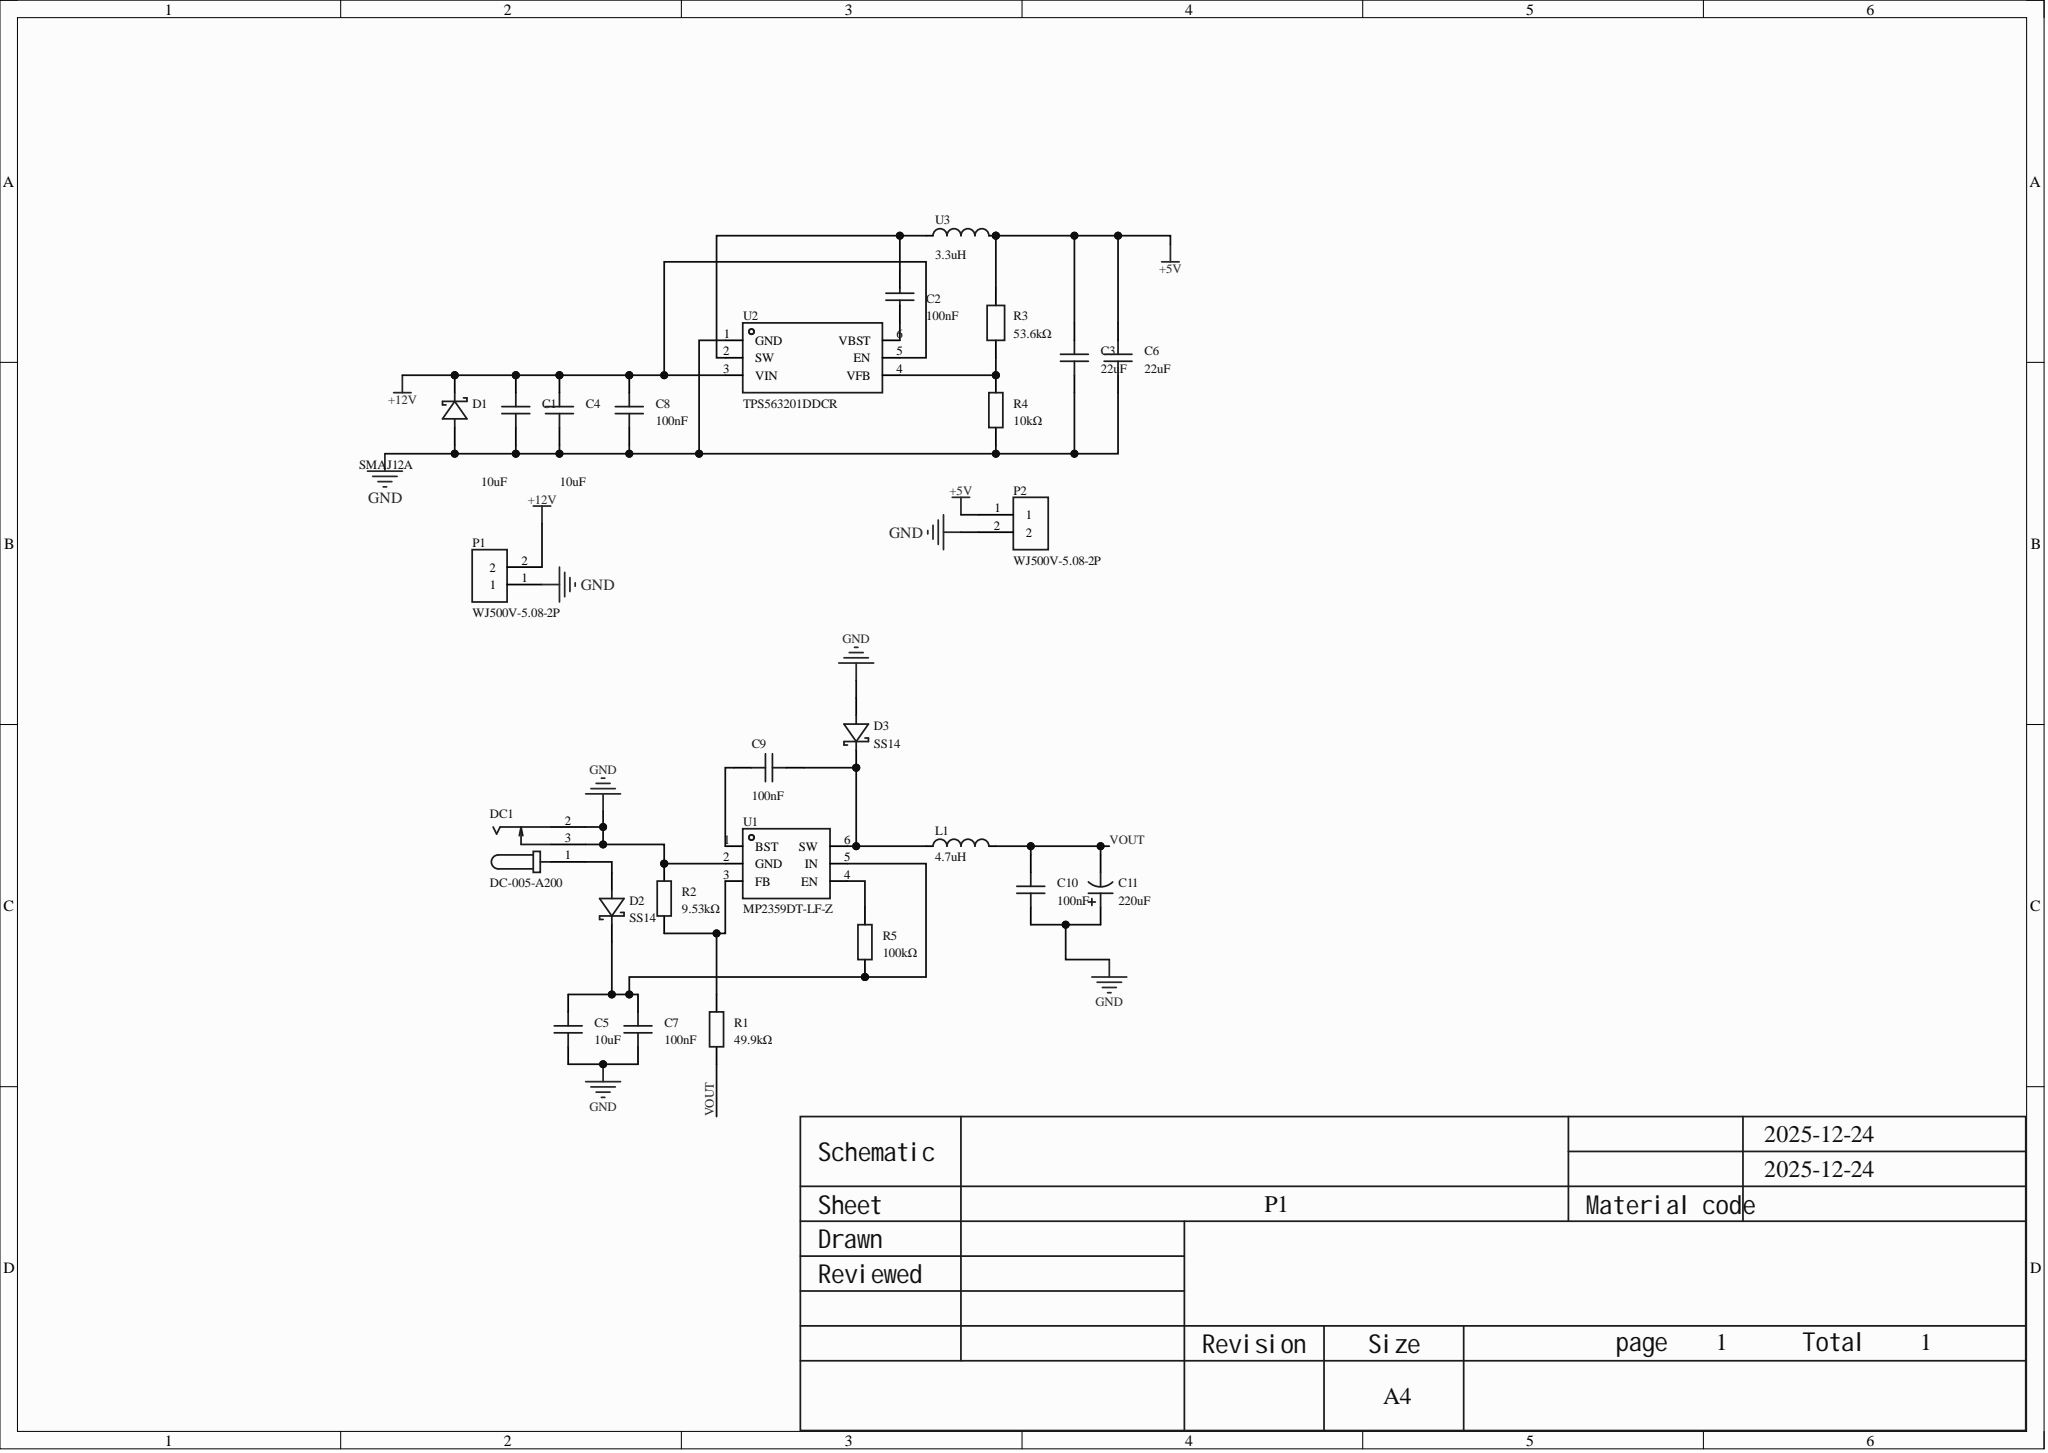Circuit board | Altium Designer | 26 parts | 13 nets
Bill of materials:
Comment,Description,Designator,Footprint,LibRef,Quantity
"10uF","Capacitance: 10uF; Tolerance: ±10%; Rated voltage: 35V; Dielectric (temp. coefficient): X5R;","C1, C4","C0805","CGA0805X5R106K350MT","2"
"100nF","Capacitance: 100nF; Tolerance: ±10%; Rated voltage: 25V; Dielectric (temp. coefficient): X7R;, Capacitance: 100nF; Tolerance: ±10%; Rated voltage: 50V; Dielectric (temp. coefficient): X7R;","C2, C7, C8, C9, C10","C0603","CL10B104KA8NNNC, CGA0603X7R104K500JT","5"
"22uF","Capacitance: 22uF; Tolerance: ±20%; Rated voltage: 10V; Dielectric (temp. coefficient): X5R;","C3, C6","C0603","HGC0603R5226M100NTHJ","2"
"10uF","Capacitance: 10uF; Tolerance: ±10%; Rated voltage: 10V; Dielectric (temp. coefficient): X5R;","C5","C0603","CGA0603X5R106K100JT","1"
"220uF","Capacitance: 220uF; Tolerance: ±20%; Rated voltage: 50V; Ripple current: 220mA@120Hz;","C11","CAP-SMD_BD10.0-L10.3-W10.3-LS11.7-FD","JVJ50V220M10x10","1"
"SMAJ12A","Reverse standoff voltage (Vrwm): 12V; Max clamping voltage: 19.9V; Peak pulse current (Ipp): 20.1A; Peak pulse power (Ppp): 400W; Breakdown voltage: 13.3V;","D1","DO-214AC_L4.3-W2.7-LS5.0-RD","SMAJ12A_C908766","1"
"SS14","Diode configuration: Single; Forward voltage (Vf): 550mV@1.0A; DC reverse voltage (Vr): 40V; Rectified current: 1A;","D2, D3","SMA_L4.3-W2.6-LS5.0-FD","SS14_C7420316","2"
"DC-005-A200","","DC1","DC-IN-TH_DC-005-A200","DC-005-A200","1"
"4.7uH","Inductance: 4.7uH; Tolerance: ±20%; Rated current: 620mA; Saturation current (Isat): -; DC resistance (DCR): 440mΩ;","L1","L0603","LQM18PN4R7MFRL","1"
"WJ500V-5.08-2P","","P1, P2","CONN-TH_2P-P5.00_WJ500V-5.08-2P","WJ500V-5.08-2P","2"
"49.9kΩ","Resistor type: Thick-film resistor; Resistance: 49.9kΩ; Tolerance: ±1%; Power: 100mW; Working voltage: 75V; Temp. coefficient: ±100ppm/?;","R1","R0603","0603WAF4992T5E","1"
"9.53kΩ","Resistor type: Thick-film resistor; Resistance: 9.53kΩ; Tolerance: ±1%; Power: 100mW; Max working voltage: 75V; Temp. coefficient: ±100ppm/?;","R2","R0603","0603WAF9531T5E","1"
"53.6kΩ","Resistor type: Thick-film resistor; Resistance: 53.6kΩ; Tolerance: ±1%; Power: 100mW; Max working voltage: 75V; Temp. coefficient: ±100ppm/?;","R3","R0603","FRC0603F5362TS","1"
"10kΩ","Resistor type: Thick-film resistor; Resistance: 10kΩ; Tolerance: ±1%; Power: 100mW; Max working voltage: 75V; Temp. coefficient: ±100ppm/?;","R4","R0603","0603WAF1002T5E","1"
"100kΩ","Resistor type: Thick-film resistor; Resistance: 100kΩ; Tolerance: ±1%; Power: 100mW; Working voltage: 75V; Temp. coefficient: ±100ppm/?;","R5","R0603","0603WAF1003T5E","1"
"MP2359DT-LF-Z","Function type: Buck; Operating voltage: 4.5V~24V; Output voltage: 810mV~15V; Output current: 1.2A; Output type: Adjustable;","U1","SOT-23-6_L2.9-W1.6-P0.95-LS2.8-BR","MP2359DT-LF-Z","1"
"TPS563201DDCR","Function type: Buck; Output type: Adjustable; Input voltage: 4.5V~17V; Output voltage: 768mV~7V; Output current: 3A;","U2","SOT-23-6_L2.9-W1.6-P0.95-LS2.8-BR","TPS563201DDCR","1"
"3.3uH","Inductance: 3.3uH; Tolerance: ±20%; Rated current: 5.3A; Saturation current (Isat): -; DC resistance (DCR): 25.4mΩ;","U3","IND-SMD_L7.4-W6.6","FDVE0630-H-3R3M=P3","1"
Netlist (Protel format):
[
C1
C0805
10uF



]
[
C2
C0603
100nF



]
[
C3
C0603
22uF



]
[
C4
C0805
10uF



]
[
C5
C0603
10uF



]
[
C6
C0603
22uF



]
[
C7
C0603
100nF



]
[
C8
C0603
100nF



]
[
C9
C0603
100nF



]
[
C10
C0603
100nF



]
[
C11
CAP-SMD_BD10.0-L10.3-W10.3-LS11.7-FD
220uF



]
[
D1
DO-214AC_L4.3-W2.7-LS5.0-RD
SMAJ12A



]
[
D2
SMA_L4.3-W2.6-LS5.0-FD
SS14



]
[
D3
SMA_L4.3-W2.6-LS5.0-FD
SS14



]
[
DC1
DC-IN-TH_DC-005-A200
DC-005-A200



]
[
L1
L0603
4.7uH



]
[
P1
CONN-TH_2P-P5.00_WJ500V-5.08-2P
WJ500V-5.08-2P



]
[
P2
CONN-TH_2P-P5.00_WJ500V-5.08-2P
WJ500V-5.08-2P



]
[
R1
R0603
49.9kΩ



]
[
R2
R0603
9.53kΩ



]
[
R3
R0603
53.6kΩ



]
[
R4
R0603
10kΩ



]
[
R5
R0603
100kΩ



]
[
U1
SOT-23-6_L2.9-W1.6-P0.95-LS2.8-BR
MP2359DT-LF-Z



]
[
U2
SOT-23-6_L2.9-W1.6-P0.95-LS2.8-BR
TPS563201DDCR



]
[
U3
IND-SMD_L7.4-W6.6
3.3uH



]
(
VOUT
C10-2
C11-2
L1-2
R1-2
)
(
NetR5_1
R5-1
U1-4
)
(
NetR3_1
R3-1
R4-2
U2-4
)
(
NetR1_1
R1-1
R2-2
U1-3
)
(
NetD2_1
D2-1
DC1-1
)
(
NetC9_2
C9-2
D3-2
L1-1
U1-6
)
(
NetC9_1
C9-1
U1-1
)
(
NetC5_2
C5-2
C7-2
D2-2
R5-2
U1-5
)
(
NetC2_2
C2-2
U2-6
)
(
NetC2_1
C2-1
U2-2
U3-1
)
(
GND
C1-1
C3-1
C4-1
C5-1
C6-1
C7-1
C8-1
C10-1
C11-1
D1-2
D3-1
DC1-2
DC1-3
P1-1
P2-2
R2-1
R4-1
U1-2
U2-1
)
(
+12V
C1-2
C4-2
C8-2
D1-1
P1-2
U2-3
U2-5
)
(
+5V
C3-2
C6-2
P2-1
R3-2
U3-2
)